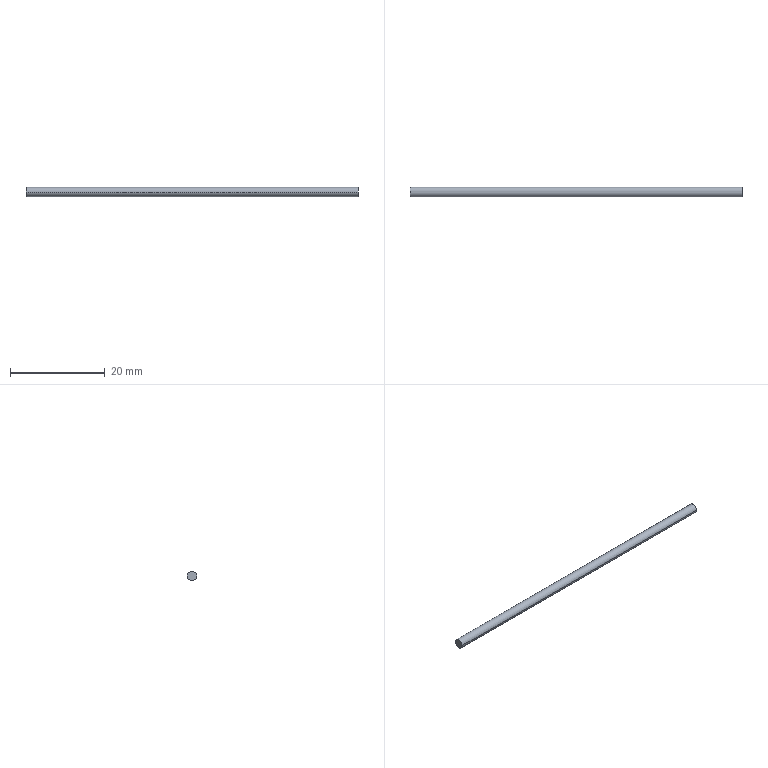Part | NX | 1 solid | 4 faces | box 70 x 2 x 2 mm | volume 219.911 mm3 | cylinder 2 | plane 2 | commonest cylinder face diameters 2 x2
STEP:
#1=CARTESIAN_POINT('',(710.,208.2,-52.5));
#2=VERTEX_POINT('',#1);
#3=CARTESIAN_POINT('',(710.,210.2,-52.5));
#4=VERTEX_POINT('',#3);
#5=CARTESIAN_POINT('',(710.,209.2,-52.5));
#6=DIRECTION('',(-1.,0.,0.));
#7=DIRECTION('',(0.,-1.,0.));
#8=AXIS2_PLACEMENT_3D('',#5,#6,#7);
#9=CIRCLE('',#8,1.);
#10=EDGE_CURVE('',#2,#4,#9,.T.);
#11=ORIENTED_EDGE('',*,*,#10,.T.);
#12=CARTESIAN_POINT('',(640.,210.2,-52.5));
#13=VERTEX_POINT('',#12);
#14=CARTESIAN_POINT('',(640.,210.2,-52.5));
#15=DIRECTION('',(-1.,0.,0.));
#16=VECTOR('',#15,1000.);
#17=LINE('',#14,#16);
#18=EDGE_CURVE('',#4,#13,#17,.T.);
#19=ORIENTED_EDGE('',*,*,#18,.T.);
#20=CARTESIAN_POINT('',(640.,208.2,-52.5));
#21=VERTEX_POINT('',#20);
#22=CARTESIAN_POINT('',(640.,209.2,-52.5));
#23=DIRECTION('',(-1.,0.,0.));
#24=DIRECTION('',(0.,-1.,0.));
#25=AXIS2_PLACEMENT_3D('',#22,#23,#24);
#26=CIRCLE('',#25,1.);
#27=EDGE_CURVE('',#21,#13,#26,.T.);
#28=ORIENTED_EDGE('',*,*,#27,.F.);
#29=CARTESIAN_POINT('',(640.,208.2,-52.5));
#30=DIRECTION('',(-1.,0.,0.));
#31=VECTOR('',#30,1000.);
#32=LINE('',#29,#31);
#33=EDGE_CURVE('',#2,#21,#32,.T.);
#34=ORIENTED_EDGE('',*,*,#33,.F.);
#35=EDGE_LOOP('',(#11,#19,#28,#34));
#36=FACE_BOUND('',#35,.T.);
#37=CARTESIAN_POINT('',(640.,209.2,-52.5));
#38=DIRECTION('',(-1.,0.,0.));
#39=DIRECTION('',(0.,-1.,0.));
#40=AXIS2_PLACEMENT_3D('',#37,#38,#39);
#41=CYLINDRICAL_SURFACE('',#40,1.);
#42=ADVANCED_FACE('',(#36),#41,.T.);
#43=CARTESIAN_POINT('',(640.,209.2,-52.5));
#44=DIRECTION('',(-1.,0.,0.));
#45=DIRECTION('',(0.,-1.,0.));
#46=AXIS2_PLACEMENT_3D('',#43,#44,#45);
#47=CIRCLE('',#46,1.);
#48=EDGE_CURVE('',#13,#21,#47,.T.);
#49=ORIENTED_EDGE('',*,*,#48,.T.);
#50=ORIENTED_EDGE('',*,*,#27,.T.);
#51=EDGE_LOOP('',(#49,#50));
#52=FACE_BOUND('',#51,.T.);
#53=CARTESIAN_POINT('',(640.,209.554,-52.627));
#54=DIRECTION('',(1.,0.,0.));
#55=DIRECTION('',(0.,-1.,0.));
#56=AXIS2_PLACEMENT_3D('',#53,#54,#55);
#57=PLANE('',#56);
#58=ADVANCED_FACE('',(#52),#57,.F.);
#59=ORIENTED_EDGE('',*,*,#10,.F.);
#60=CARTESIAN_POINT('',(710.,209.2,-52.5));
#61=DIRECTION('',(-1.,0.,0.));
#62=DIRECTION('',(0.,-1.,0.));
#63=AXIS2_PLACEMENT_3D('',#60,#61,#62);
#64=CIRCLE('',#63,1.);
#65=EDGE_CURVE('',#4,#2,#64,.T.);
#66=ORIENTED_EDGE('',*,*,#65,.F.);
#67=EDGE_LOOP('',(#59,#66));
#68=FACE_BOUND('',#67,.T.);
#69=CARTESIAN_POINT('',(710.,209.554,-52.627));
#70=DIRECTION('',(1.,0.,0.));
#71=DIRECTION('',(0.,-1.,0.));
#72=AXIS2_PLACEMENT_3D('',#69,#70,#71);
#73=PLANE('',#72);
#74=ADVANCED_FACE('',(#68),#73,.T.);
#75=ORIENTED_EDGE('',*,*,#48,.F.);
#76=ORIENTED_EDGE('',*,*,#18,.F.);
#77=ORIENTED_EDGE('',*,*,#65,.T.);
#78=ORIENTED_EDGE('',*,*,#33,.T.);
#79=EDGE_LOOP('',(#75,#76,#77,#78));
#80=FACE_BOUND('',#79,.T.);
#81=CARTESIAN_POINT('',(640.,209.2,-52.5));
#82=DIRECTION('',(-1.,0.,0.));
#83=DIRECTION('',(0.,-1.,0.));
#84=AXIS2_PLACEMENT_3D('',#81,#82,#83);
#85=CYLINDRICAL_SURFACE('',#84,1.);
#86=ADVANCED_FACE('',(#80),#85,.T.);
#87=CLOSED_SHELL('',(#42,#58,#74,#86));
#88=MANIFOLD_SOLID_BREP('',#87);
#89=(LENGTH_UNIT()NAMED_UNIT(*)SI_UNIT(.MILLI.,.METRE.));
#90=UNCERTAINTY_MEASURE_WITH_UNIT(LENGTH_MEASURE(0.00001),#89,'','');
#91=(NAMED_UNIT(*)PLANE_ANGLE_UNIT()SI_UNIT($,.RADIAN.));
#92=(NAMED_UNIT(*)SI_UNIT($,.STERADIAN.)SOLID_ANGLE_UNIT());
#93=(GEOMETRIC_REPRESENTATION_CONTEXT(3)GLOBAL_UNCERTAINTY_ASSIGNED_CONTEXT((#90))GLOBAL_UNIT_ASSIGNED_CONTEXT((#89,#91,#92))REPRESENTATION_CONTEXT('',''));
#94=ADVANCED_BREP_SHAPE_REPRESENTATION('',(#88),#93);